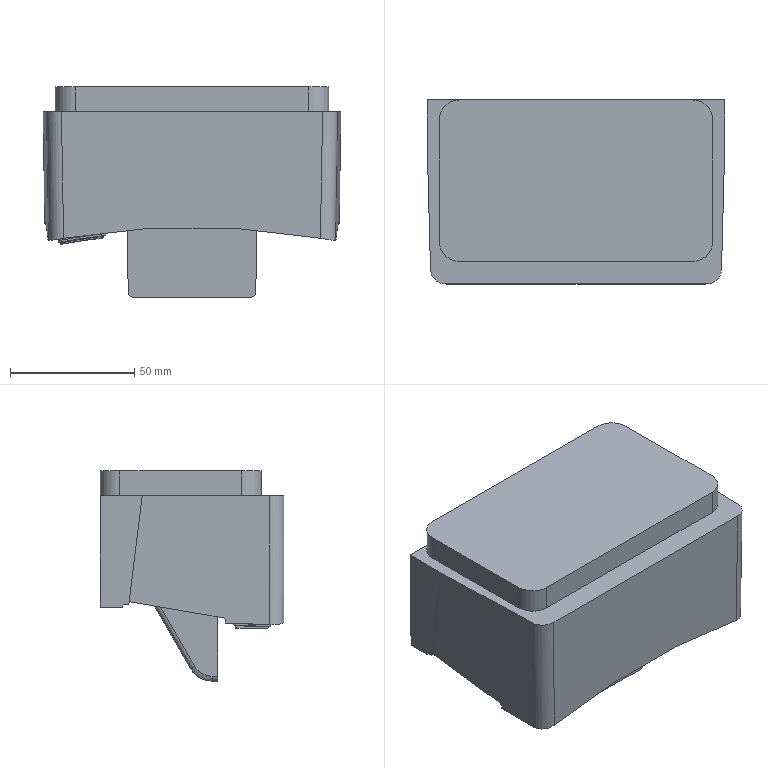Part | STEP file | 1 solid | 101 faces | box 119.805 x 74.045 x 84.64 mm | volume 483562 mm3 | plane 43 | spline 29 | cylinder 23 | torus 4 | cone 2 | commonest cylinder face diameters 1.005 x8 3.015 x4 4.02 x4 16 x4 12 x2 20.1 x1